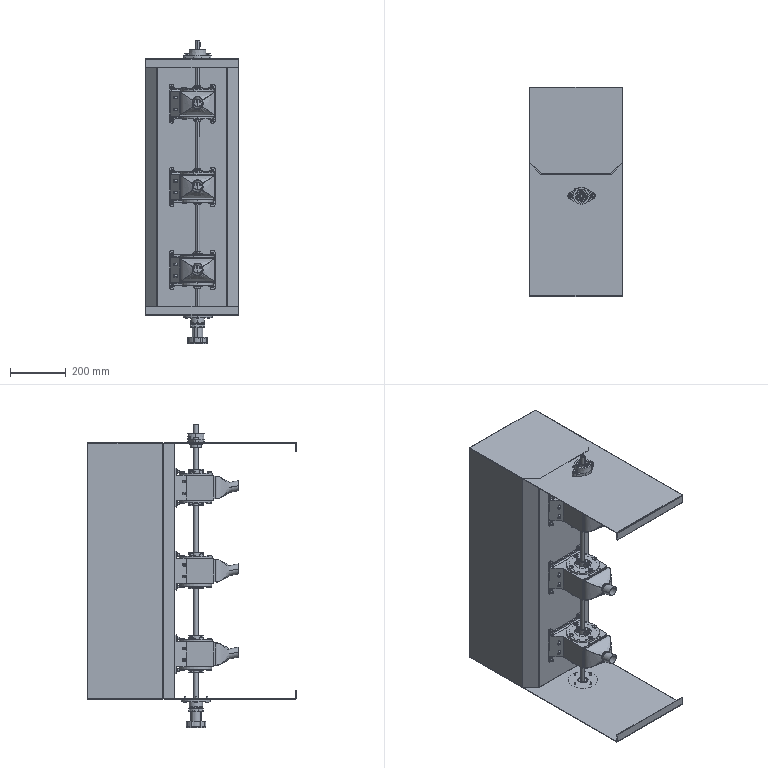Part | SolidWorks | features ReferencePattern 29, LocalLPattern 4, CompositeCurve 2, MirrorCompFeat 2, LocalCirPattern 1 | 122 solids | 7218 faces | volume 6401215 mm3 | plane 5232 | cylinder 1075 | cone 602 | torus 191 | spline 96 | sphere 22 | commonest cylinder face diameters 8 x264 6 x114 100 x63 10 x61 5 x58 4 x48